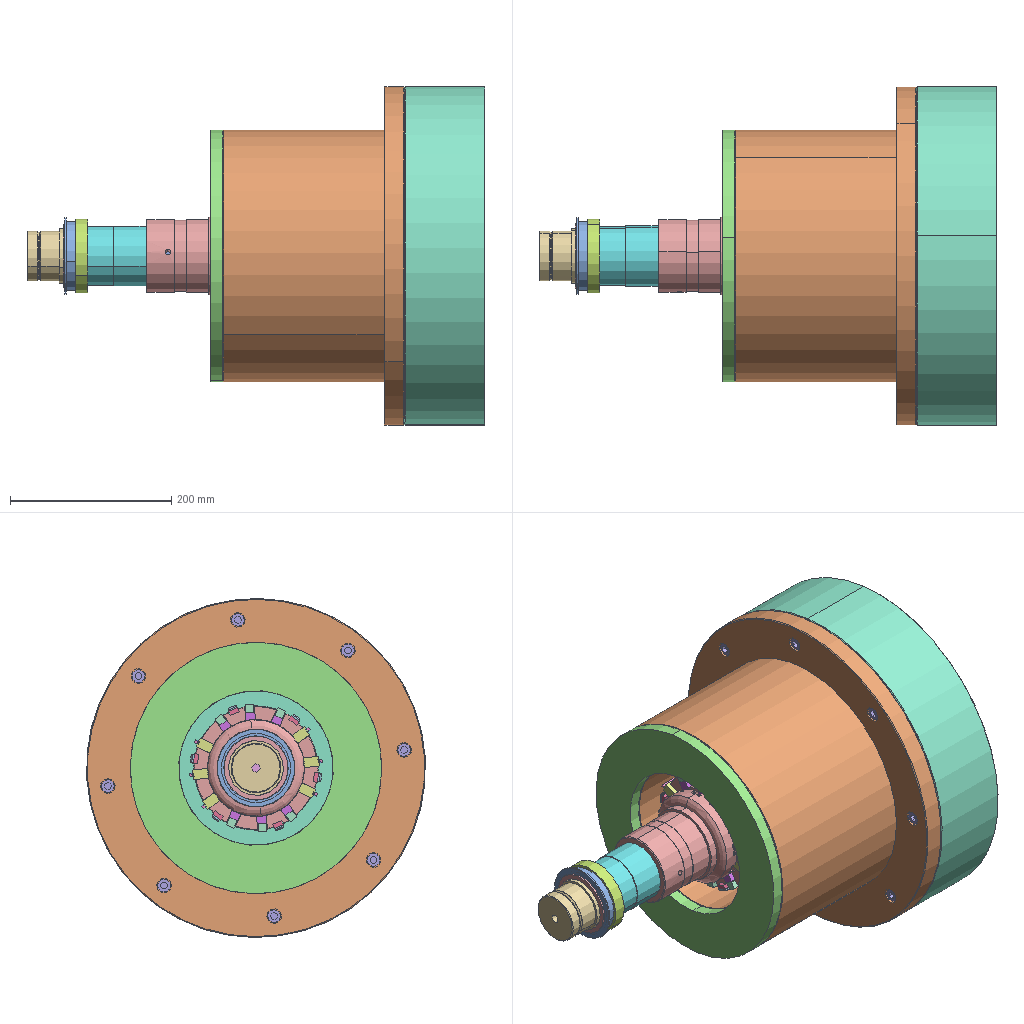Assembly | SolidWorks | 29 different items | 67 placed | box 568 x 420 x 420 mm
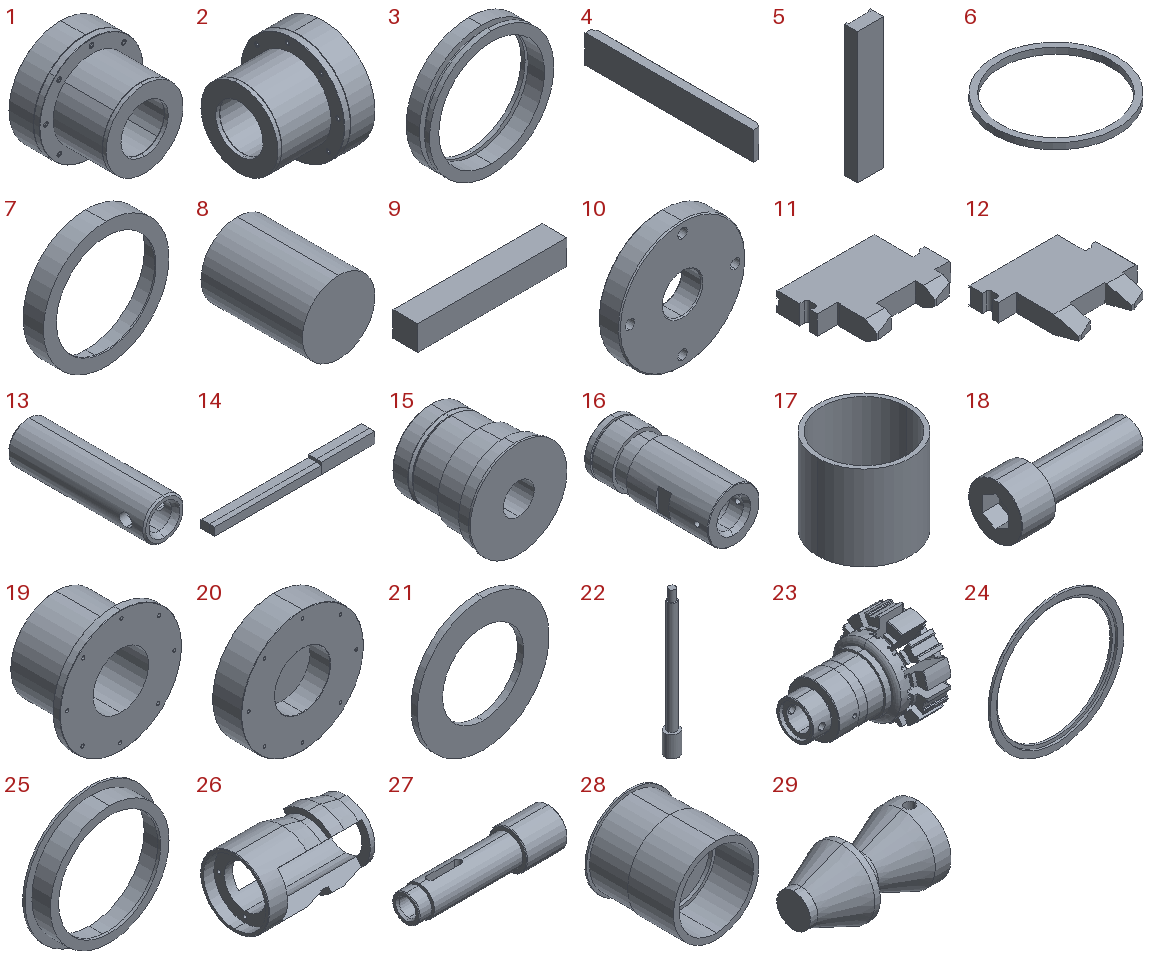Parts list (item | name | quantity | parent item | size | volume | features):
1 | (subassembly) | x1 | in 2 | 420 x 340 x 420 mm | 19334956 mm3 | features ReferencePattern 7, LocalCirPattern 1
2 | (subassembly) | x1 | - | 340 x 420 x 420 mm | 19334956 mm3 | -
3 | - | x1 | - | 80 x 15 x 80 mm | 16407 mm3 | features Revolution 1
4 | - | x6 | - | 4 x 60 x 10 mm | 2276 mm3 | features Chamfer 2, Extrusion 1
5 | - | x6 | - | 12 x 6 x 60 mm | 3870 mm3 | features Extrusion 1, ICE 1
6 | - | x1 | - | 60 x 60 x 3 mm | 1612 mm3 | features Extrusion 1
7 | - | x1 | - | 92 x 15 x 92 mm | 14205 mm3 | features Revolution 1
8 | - | x1 | - | 25 x 35 x 25 mm | 17181 mm3 | features Revolution 1
9 | - | x6 | - | 60 x 10 x 10 mm | 6000 mm3 | features Extrusion 1
10 | - | x1 | - | 60 x 10 x 60 mm | 24256 mm3 | features HoleWzd 2, Chamfer 1, Extrusion 1
11 | - | x6 | - | 70 x 49.5 x 12 mm | 28944 mm3 | features ICE 2, Chamfer 1, Extrusion 1
12 | - | x6 | - | 70 x 62.5 x 12 mm | 33880 mm3 | features ICE 2, Chamfer 1, Extrusion 1
13 | - | x1 | - | 13 x 44 x 13 mm | 3507 mm3 | features Chamfer 2, 3DProfileFeature 1, Extrusion 1, HoleWzd 1
14 | - | x6 | - | 60 x 5 x 4 mm | 1000 mm3 | features ICE 3, Extrusion 1
15 | - | x1 | - | 78 x 71.5 x 78 mm | 226793 mm3 | features Chamfer 1, Revolution 1
16 | - | x1 | - | 40 x 95 x 40 mm | 59618 mm3 | features Chamfer 2, ICE 2, 3DProfileFeature 1, Extrusion 1, HoleWzd 1, RevCut 1
17 | - | x1 | - | 220 x 220 x 200 mm | 1319469 mm3 | features ExtruThin 1
18 | - | x8 | in 1 | 40 x 16 x 16 mm | 4081 mm3 | features BlendCut 1, Cut 1, Fillet 1, LPattern 1, RevCut 1, Revolution 1
19 | - | x1 | in 1 | 420 x 225 x 420 mm | 6770057 mm3 | features ICE 3, Chamfer 1, CirPattern 1, Extrusion 1, HoleWzd 1
20 | - | x1 | in 1 | 420 x 100 x 420 mm | 11820755 mm3 | features Chamfer 1, CirPattern 1, Extrusion 1, HoleWzd 1, ICE 1
21 | - | x1 | in 1 | 311.64 x 15 x 311.64 mm | 711495 mm3 | features Extrusion 1
22 | - | x1 | - | 13 x 13 x 135 mm | 8178 mm3 | features ICE 2, Chamfer 1, Extrusion 1, HoleWzd 1
23 | - | x1 | - | 209 x 153.532 x 153.532 mm | 1079981 mm3 | features ICE 9, 3DProfileFeature 6, CirPattern 6, HoleWzd 6, Chamfer 2, RefAxis 1, RevCut 1, Revolution 1
24 | - | x2 | - | 86 x 3 x 86 mm | 3016 mm3 | features Revolution 1
25 | - | x1 | - | 96 x 15 x 96 mm | 15329 mm3 | features Revolution 1
26 | - | x1 | - | 107 x 66 x 66 mm | 107081 mm3 | features Chamfer 1, HoleWzd 1, MirrorPattern 1, RefAxis 1, RevCut 1, Revolution 1
27 | - | x1 | - | 105 x 28 x 28 mm | 30891 mm3 | features ICE 3, Chamfer 2, Extrusion 1, HoleWzd 1, RevCut 1
28 | - | x1 | - | 78 x 76 x 78 mm | 183588 mm3 | features Revolution 1
29 | - | x1 | - | 74 x 40 x 40 mm | 56034 mm3 | features HoleWzd 2, 3DProfileFeature 1, Chamfer 1, Revolution 1
Mates (type | each side: item.copy, entity, surface, feature):
In the top assembly
Coincident | 23.1 face plane Revolve 1 | 11.1 face plane Boss-Extrude 1
Coincident | 23.1 face plane CirPattern 6 | 11.1 face plane Boss-Extrude 1
Coincident | 23.1 face plane CirPattern 6 | 12.1 face plane Boss-Extrude 1
Coincident | 23.1 face plane Revolve 1 | 12.1 face plane Boss-Extrude 1
Coincident | 23.1 face plane CirPattern 9 | 5.1 face plane Boss-Extrude 1 | 2 times
Coincident | 11.2 face plane Boss-Extrude 1 | 5.1 face plane Boss-Extrude 1
Coincident | 5.1 face plane Cut-Extrude 1 | 4.1 face plane Boss-Extrude 1 | 2 times
Coincident | 5.1 face plane Boss-Extrude 1 | 4.1 face plane Boss-Extrude 1
Coincident | 12.1 face plane Cut-Extrude 2 | 9.1 face plane Boss-Extrude 1 | 2 times
Coincident | 12.1 face plane Boss-Extrude 1 | 9.1 face plane Boss-Extrude 1
Coincident | 11.1 face plane Cut-Extrude 2 | 14.1 face plane Boss-Extrude 1 | 2 times
Coincident | 11.1 face plane Boss-Extrude 1 | 14.1 face plane Boss-Extrude 1
Concentric | 16.1 face cylinder Boss-Extrude 1 | 27.1 face cylinder Boss-Extrude 1
Concentric | 16.1 face cylinder Boss-Extrude 1 | 22.1 face cylinder Boss-Extrude 1
Coincident | 16.1 face plane Boss-Extrude 1 | 27.1 face plane Boss-Extrude 1
Concentric | 16.1 face cylinder Boss-Extrude 1 | 10.1 face cylinder Boss-Extrude 1
Coincident | 16.1 face plane Boss-Extrude 1 | 10.1 face plane Boss-Extrude 1
Coincident | 23.1 face plane Revolve 1 | 16.1 face plane Boss-Extrude 1
Concentric | 23.1 face cylinder Revolve 1 | 16.1 face cylinder Boss-Extrude 1
Concentric | 23.1 face cylinder Cut-Extrude 1 | 26.1 face cylinder Revolve 1
Concentric | 26.1 face cylinder Revolve 1 | 13.1 face cylinder Boss-Extrude 1
Concentric | 16.1 face cylinder Ø4.0 (4) DiameterHole 3 | 13.1 face cylinder Ø4.0 (4) DiameterHole 1
Concentric | 10.1 face cylinder HoleSize(%per)Socket Head CapScrewtype1 | 26.1 face cylinder M4 Tapped Hole 1
Parallel | 16.1 face cylinder Ø4.0 (4) DiameterHole 3 | 27.1 face cylinder Cut-Extrude 2
Parallel | 12.1 face plane Cut-Extrude 1 | 26.1 face plane Mirror 1
Coincident | 23.1 plane | 27.1 plane
Concentric | 22.1 face cylinder Boss-Extrude 2 | 29.1 face cylinder M6 Tapped Hole 1
Coincident | 22.1 face plane Boss-Extrude 2 | 29.1 face plane Revolve 1
Coincident | 29.1 face cone Revolve 1 | 12.2 vertex
Coincident | 26.1 face cone Revolve 1 | 11.1 vertex
DistanceDim | 10.1 face plane Boss-Extrude 1 | 22.1 face plane Boss-Extrude 1
DistanceDim | 26.1 face plane Revolve 1 | 16.1 face plane Boss-Extrude 1
Concentric | 23.1 face cylinder Revolve 1 | 28.1 face cylinder Revolve 1
Coincident | 23.1 face plane Revolve 1 | 28.1 face plane Revolve 1
Coincident | 23.1 face plane Revolve 1 | 6.1 face plane Boss-Extrude 1
Concentric | 19.1 face cylinder Boss-Extrude 2 | 23.1 face cylinder Revolve 1
DistanceDim | 21.1 face plane Boss-Extrude 1 | 23.1 face plane Revolve 1
In subassembly 1
Coincident | 20.1 face plane Boss-Extrude 1 | 19.2 face plane Boss-Extrude 1
Concentric | 20.1 face cylinder Boss-Extrude 1 | 19.2 face cylinder Boss-Extrude 2
Concentric | 19.2 face cylinder CirPattern 2 | 18.1 face cylinder Base-Revolve
Coincident | 19.2 face plane CirPattern 2 | 18.1 face plane Base-Revolve
Concentric | 20.1 face cylinder CirPattern 1 | 18.2 face cylinder Base-Revolve
Concentric | 19.2 face cylinder Boss-Extrude 2 | 21.2 face cylinder Boss-Extrude 1
Coincident | 19.2 face plane Boss-Extrude 2 | 21.2 face plane Boss-Extrude 1